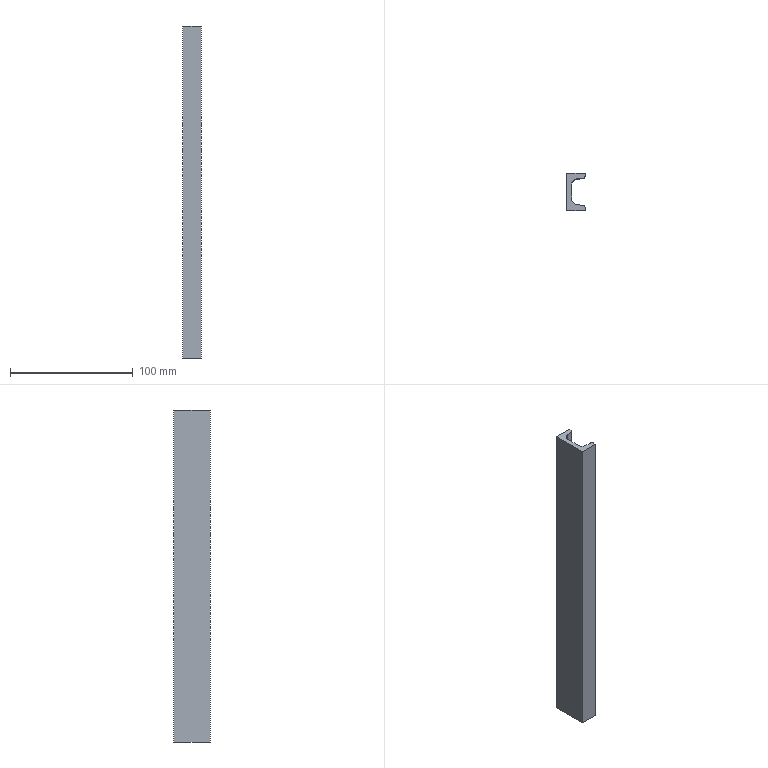Part | STEP file | DIN 1026-1 U 30x15 1785507675476 | 1 solid | 14 faces | box 15 x 30 x 270 mm | volume 59739 mm3 | plane 10 | cylinder 4 | commonest cylinder face diameters 4 x2 9 x2
STEP:
#1=CARTESIAN_POINT('',(4.,-6.066,270.));
#2=VERTEX_POINT('',#1);
#3=CARTESIAN_POINT('',(8.141,-10.551,270.));
#4=VERTEX_POINT('',#3);
#5=CARTESIAN_POINT('',(8.5,-6.066,270.));
#6=DIRECTION('',(0.,0.,1.));
#7=DIRECTION('',(-1.,0.,0.));
#8=AXIS2_PLACEMENT_3D('',#5,#6,#7);
#9=CIRCLE('',#8,4.5);
#10=EDGE_CURVE('',#2,#4,#9,.T.);
#11=ORIENTED_EDGE('',*,*,#10,.T.);
#12=CARTESIAN_POINT('',(8.141,-10.551,0.));
#13=VERTEX_POINT('',#12);
#14=CARTESIAN_POINT('',(8.141,-10.551,0.));
#15=DIRECTION('',(0.,0.,1.));
#16=VECTOR('',#15,10.);
#17=LINE('',#14,#16);
#18=EDGE_CURVE('',#13,#4,#17,.T.);
#19=ORIENTED_EDGE('',*,*,#18,.F.);
#20=CARTESIAN_POINT('',(4.,-6.066,0.));
#21=VERTEX_POINT('',#20);
#22=CARTESIAN_POINT('',(8.5,-6.066,0.));
#23=DIRECTION('',(0.,0.,1.));
#24=DIRECTION('',(-1.,0.,0.));
#25=AXIS2_PLACEMENT_3D('',#22,#23,#24);
#26=CIRCLE('',#25,4.5);
#27=EDGE_CURVE('',#21,#13,#26,.T.);
#28=ORIENTED_EDGE('',*,*,#27,.F.);
#29=CARTESIAN_POINT('',(4.,-6.066,0.));
#30=DIRECTION('',(0.,0.,1.));
#31=VECTOR('',#30,10.);
#32=LINE('',#29,#31);
#33=EDGE_CURVE('',#21,#2,#32,.T.);
#34=ORIENTED_EDGE('',*,*,#33,.T.);
#35=EDGE_LOOP('',(#11,#19,#28,#34));
#36=FACE_OUTER_BOUND('',#35,.T.);
#37=CARTESIAN_POINT('',(8.5,-6.066,0.));
#38=DIRECTION('',(0.,0.,1.));
#39=DIRECTION('',(-1.,0.,0.));
#40=AXIS2_PLACEMENT_3D('',#37,#38,#39);
#41=CYLINDRICAL_SURFACE('',#40,4.5);
#42=ADVANCED_FACE('',(#36),#41,.F.);
#43=CARTESIAN_POINT('',(13.159,-10.953,270.));
#44=VERTEX_POINT('',#43);
#45=CARTESIAN_POINT('',(7.403,-10.492,270.));
#46=DIRECTION('',(0.9968,-0.07975,0.));
#47=VECTOR('',#46,10.);
#48=LINE('',#45,#47);
#49=EDGE_CURVE('',#4,#44,#48,.T.);
#50=ORIENTED_EDGE('',*,*,#49,.T.);
#51=CARTESIAN_POINT('',(13.159,-10.953,0.));
#52=VERTEX_POINT('',#51);
#53=CARTESIAN_POINT('',(13.159,-10.953,0.));
#54=DIRECTION('',(0.,0.,1.));
#55=VECTOR('',#54,10.);
#56=LINE('',#53,#55);
#57=EDGE_CURVE('',#52,#44,#56,.T.);
#58=ORIENTED_EDGE('',*,*,#57,.F.);
#59=CARTESIAN_POINT('',(7.403,-10.492,0.));
#60=DIRECTION('',(0.9968,-0.07975,0.));
#61=VECTOR('',#60,10.);
#62=LINE('',#59,#61);
#63=EDGE_CURVE('',#13,#52,#62,.T.);
#64=ORIENTED_EDGE('',*,*,#63,.F.);
#65=ORIENTED_EDGE('',*,*,#18,.T.);
#66=EDGE_LOOP('',(#50,#58,#64,#65));
#67=FACE_OUTER_BOUND('',#66,.T.);
#68=CARTESIAN_POINT('',(8.141,-10.551,0.));
#69=DIRECTION('',(0.07975,0.9968,0.));
#70=DIRECTION('',(0.,0.,1.));
#71=AXIS2_PLACEMENT_3D('',#68,#69,#70);
#72=PLANE('',#71);
#73=ADVANCED_FACE('',(#67),#72,.T.);
#74=CARTESIAN_POINT('',(15.,-12.946,270.));
#75=VERTEX_POINT('',#74);
#76=CARTESIAN_POINT('',(13.,-12.946,270.));
#77=DIRECTION('',(0.,0.,-1.));
#78=DIRECTION('',(-1.,0.,0.));
#79=AXIS2_PLACEMENT_3D('',#76,#77,#78);
#80=CIRCLE('',#79,2.);
#81=EDGE_CURVE('',#44,#75,#80,.T.);
#82=ORIENTED_EDGE('',*,*,#81,.T.);
#83=CARTESIAN_POINT('',(15.,-12.946,0.));
#84=VERTEX_POINT('',#83);
#85=CARTESIAN_POINT('',(15.,-12.946,0.));
#86=DIRECTION('',(0.,0.,1.));
#87=VECTOR('',#86,10.);
#88=LINE('',#85,#87);
#89=EDGE_CURVE('',#84,#75,#88,.T.);
#90=ORIENTED_EDGE('',*,*,#89,.F.);
#91=CARTESIAN_POINT('',(13.,-12.946,0.));
#92=DIRECTION('',(0.,0.,-1.));
#93=DIRECTION('',(-1.,0.,0.));
#94=AXIS2_PLACEMENT_3D('',#91,#92,#93);
#95=CIRCLE('',#94,2.);
#96=EDGE_CURVE('',#52,#84,#95,.T.);
#97=ORIENTED_EDGE('',*,*,#96,.F.);
#98=ORIENTED_EDGE('',*,*,#57,.T.);
#99=EDGE_LOOP('',(#82,#90,#97,#98));
#100=FACE_OUTER_BOUND('',#99,.T.);
#101=CARTESIAN_POINT('',(13.,-12.946,0.));
#102=DIRECTION('',(0.,0.,1.));
#103=DIRECTION('',(-1.,0.,0.));
#104=AXIS2_PLACEMENT_3D('',#101,#102,#103);
#105=CYLINDRICAL_SURFACE('',#104,2.);
#106=ADVANCED_FACE('',(#100),#105,.T.);
#107=CARTESIAN_POINT('',(15.,-15.,270.));
#108=VERTEX_POINT('',#107);
#109=CARTESIAN_POINT('',(15.,-6.473,270.));
#110=DIRECTION('',(0.,-1.,0.));
#111=VECTOR('',#110,10.);
#112=LINE('',#109,#111);
#113=EDGE_CURVE('',#75,#108,#112,.T.);
#114=ORIENTED_EDGE('',*,*,#113,.T.);
#115=CARTESIAN_POINT('',(15.,-15.,0.));
#116=VERTEX_POINT('',#115);
#117=CARTESIAN_POINT('',(15.,-15.,0.));
#118=DIRECTION('',(0.,0.,1.));
#119=VECTOR('',#118,10.);
#120=LINE('',#117,#119);
#121=EDGE_CURVE('',#116,#108,#120,.T.);
#122=ORIENTED_EDGE('',*,*,#121,.F.);
#123=CARTESIAN_POINT('',(15.,-6.473,0.));
#124=DIRECTION('',(0.,-1.,0.));
#125=VECTOR('',#124,10.);
#126=LINE('',#123,#125);
#127=EDGE_CURVE('',#84,#116,#126,.T.);
#128=ORIENTED_EDGE('',*,*,#127,.F.);
#129=ORIENTED_EDGE('',*,*,#89,.T.);
#130=EDGE_LOOP('',(#114,#122,#128,#129));
#131=FACE_OUTER_BOUND('',#130,.T.);
#132=CARTESIAN_POINT('',(15.,-12.946,0.));
#133=DIRECTION('',(1.,0.,0.));
#134=DIRECTION('',(0.,0.,-1.));
#135=AXIS2_PLACEMENT_3D('',#132,#133,#134);
#136=PLANE('',#135);
#137=ADVANCED_FACE('',(#131),#136,.T.);
#138=CARTESIAN_POINT('',(0.,-15.,270.));
#139=VERTEX_POINT('',#138);
#140=CARTESIAN_POINT('',(11.25,-15.,270.));
#141=DIRECTION('',(-1.,0.,0.));
#142=VECTOR('',#141,10.);
#143=LINE('',#140,#142);
#144=EDGE_CURVE('',#108,#139,#143,.T.);
#145=ORIENTED_EDGE('',*,*,#144,.T.);
#146=CARTESIAN_POINT('',(0.,-15.,0.));
#147=VERTEX_POINT('',#146);
#148=CARTESIAN_POINT('',(0.,-15.,0.));
#149=DIRECTION('',(0.,0.,1.));
#150=VECTOR('',#149,10.);
#151=LINE('',#148,#150);
#152=EDGE_CURVE('',#147,#139,#151,.T.);
#153=ORIENTED_EDGE('',*,*,#152,.F.);
#154=CARTESIAN_POINT('',(11.25,-15.,0.));
#155=DIRECTION('',(-1.,0.,0.));
#156=VECTOR('',#155,10.);
#157=LINE('',#154,#156);
#158=EDGE_CURVE('',#116,#147,#157,.T.);
#159=ORIENTED_EDGE('',*,*,#158,.F.);
#160=ORIENTED_EDGE('',*,*,#121,.T.);
#161=EDGE_LOOP('',(#145,#153,#159,#160));
#162=FACE_OUTER_BOUND('',#161,.T.);
#163=CARTESIAN_POINT('',(15.,-15.,0.));
#164=DIRECTION('',(0.,-1.,0.));
#165=DIRECTION('',(0.,0.,-1.));
#166=AXIS2_PLACEMENT_3D('',#163,#164,#165);
#167=PLANE('',#166);
#168=ADVANCED_FACE('',(#162),#167,.T.);
#169=CARTESIAN_POINT('',(0.,15.,270.));
#170=VERTEX_POINT('',#169);
#171=CARTESIAN_POINT('',(0.,0.,270.));
#172=DIRECTION('',(0.,1.,0.));
#173=VECTOR('',#172,10.);
#174=LINE('',#171,#173);
#175=EDGE_CURVE('',#139,#170,#174,.T.);
#176=ORIENTED_EDGE('',*,*,#175,.T.);
#177=CARTESIAN_POINT('',(0.,15.,0.));
#178=VERTEX_POINT('',#177);
#179=CARTESIAN_POINT('',(0.,15.,0.));
#180=DIRECTION('',(0.,0.,1.));
#181=VECTOR('',#180,10.);
#182=LINE('',#179,#181);
#183=EDGE_CURVE('',#178,#170,#182,.T.);
#184=ORIENTED_EDGE('',*,*,#183,.F.);
#185=CARTESIAN_POINT('',(0.,0.,0.));
#186=DIRECTION('',(0.,1.,0.));
#187=VECTOR('',#186,10.);
#188=LINE('',#185,#187);
#189=EDGE_CURVE('',#147,#178,#188,.T.);
#190=ORIENTED_EDGE('',*,*,#189,.F.);
#191=ORIENTED_EDGE('',*,*,#152,.T.);
#192=EDGE_LOOP('',(#176,#184,#190,#191));
#193=FACE_OUTER_BOUND('',#192,.T.);
#194=CARTESIAN_POINT('',(0.,0.,0.));
#195=DIRECTION('',(-1.,0.,0.));
#196=DIRECTION('',(0.,0.,1.));
#197=AXIS2_PLACEMENT_3D('',#194,#195,#196);
#198=PLANE('',#197);
#199=ADVANCED_FACE('',(#193),#198,.T.);
#200=CARTESIAN_POINT('',(15.,15.,270.));
#201=VERTEX_POINT('',#200);
#202=CARTESIAN_POINT('',(3.75,15.,270.));
#203=DIRECTION('',(1.,0.,0.));
#204=VECTOR('',#203,10.);
#205=LINE('',#202,#204);
#206=EDGE_CURVE('',#170,#201,#205,.T.);
#207=ORIENTED_EDGE('',*,*,#206,.T.);
#208=CARTESIAN_POINT('',(15.,15.,0.));
#209=VERTEX_POINT('',#208);
#210=CARTESIAN_POINT('',(15.,15.,0.));
#211=DIRECTION('',(0.,0.,1.));
#212=VECTOR('',#211,10.);
#213=LINE('',#210,#212);
#214=EDGE_CURVE('',#209,#201,#213,.T.);
#215=ORIENTED_EDGE('',*,*,#214,.F.);
#216=CARTESIAN_POINT('',(3.75,15.,0.));
#217=DIRECTION('',(1.,0.,0.));
#218=VECTOR('',#217,10.);
#219=LINE('',#216,#218);
#220=EDGE_CURVE('',#178,#209,#219,.T.);
#221=ORIENTED_EDGE('',*,*,#220,.F.);
#222=ORIENTED_EDGE('',*,*,#183,.T.);
#223=EDGE_LOOP('',(#207,#215,#221,#222));
#224=FACE_OUTER_BOUND('',#223,.T.);
#225=CARTESIAN_POINT('',(0.,15.,0.));
#226=DIRECTION('',(0.,1.,0.));
#227=DIRECTION('',(0.,0.,1.));
#228=AXIS2_PLACEMENT_3D('',#225,#226,#227);
#229=PLANE('',#228);
#230=ADVANCED_FACE('',(#224),#229,.T.);
#231=CARTESIAN_POINT('',(15.,12.946,270.));
#232=VERTEX_POINT('',#231);
#233=CARTESIAN_POINT('',(15.,7.5,270.));
#234=DIRECTION('',(0.,-1.,0.));
#235=VECTOR('',#234,10.);
#236=LINE('',#233,#235);
#237=EDGE_CURVE('',#201,#232,#236,.T.);
#238=ORIENTED_EDGE('',*,*,#237,.T.);
#239=CARTESIAN_POINT('',(15.,12.946,0.));
#240=VERTEX_POINT('',#239);
#241=CARTESIAN_POINT('',(15.,12.946,0.));
#242=DIRECTION('',(0.,0.,1.));
#243=VECTOR('',#242,10.);
#244=LINE('',#241,#243);
#245=EDGE_CURVE('',#240,#232,#244,.T.);
#246=ORIENTED_EDGE('',*,*,#245,.F.);
#247=CARTESIAN_POINT('',(15.,7.5,0.));
#248=DIRECTION('',(0.,-1.,0.));
#249=VECTOR('',#248,10.);
#250=LINE('',#247,#249);
#251=EDGE_CURVE('',#209,#240,#250,.T.);
#252=ORIENTED_EDGE('',*,*,#251,.F.);
#253=ORIENTED_EDGE('',*,*,#214,.T.);
#254=EDGE_LOOP('',(#238,#246,#252,#253));
#255=FACE_OUTER_BOUND('',#254,.T.);
#256=CARTESIAN_POINT('',(15.,15.,0.));
#257=DIRECTION('',(1.,0.,0.));
#258=DIRECTION('',(0.,0.,-1.));
#259=AXIS2_PLACEMENT_3D('',#256,#257,#258);
#260=PLANE('',#259);
#261=ADVANCED_FACE('',(#255),#260,.T.);
#262=CARTESIAN_POINT('',(13.159,10.953,270.));
#263=VERTEX_POINT('',#262);
#264=CARTESIAN_POINT('',(13.,12.946,270.));
#265=DIRECTION('',(0.,0.,-1.));
#266=DIRECTION('',(-0.07975,0.9968,0.));
#267=AXIS2_PLACEMENT_3D('',#264,#265,#266);
#268=CIRCLE('',#267,2.);
#269=EDGE_CURVE('',#232,#263,#268,.T.);
#270=ORIENTED_EDGE('',*,*,#269,.T.);
#271=CARTESIAN_POINT('',(13.159,10.953,0.));
#272=VERTEX_POINT('',#271);
#273=CARTESIAN_POINT('',(13.159,10.953,0.));
#274=DIRECTION('',(0.,0.,1.));
#275=VECTOR('',#274,10.);
#276=LINE('',#273,#275);
#277=EDGE_CURVE('',#272,#263,#276,.T.);
#278=ORIENTED_EDGE('',*,*,#277,.F.);
#279=CARTESIAN_POINT('',(13.,12.946,0.));
#280=DIRECTION('',(0.,0.,-1.));
#281=DIRECTION('',(-0.07975,0.9968,0.));
#282=AXIS2_PLACEMENT_3D('',#279,#280,#281);
#283=CIRCLE('',#282,2.);
#284=EDGE_CURVE('',#240,#272,#283,.T.);
#285=ORIENTED_EDGE('',*,*,#284,.F.);
#286=ORIENTED_EDGE('',*,*,#245,.T.);
#287=EDGE_LOOP('',(#270,#278,#285,#286));
#288=FACE_OUTER_BOUND('',#287,.T.);
#289=CARTESIAN_POINT('',(13.,12.946,0.));
#290=DIRECTION('',(0.,0.,1.));
#291=DIRECTION('',(-0.07975,0.9968,0.));
#292=AXIS2_PLACEMENT_3D('',#289,#290,#291);
#293=CYLINDRICAL_SURFACE('',#292,2.);
#294=ADVANCED_FACE('',(#288),#293,.T.);
#295=CARTESIAN_POINT('',(8.141,10.551,270.));
#296=VERTEX_POINT('',#295);
#297=CARTESIAN_POINT('',(9.912,10.693,270.));
#298=DIRECTION('',(-0.9968,-0.07975,0.));
#299=VECTOR('',#298,10.);
#300=LINE('',#297,#299);
#301=EDGE_CURVE('',#263,#296,#300,.T.);
#302=ORIENTED_EDGE('',*,*,#301,.T.);
#303=CARTESIAN_POINT('',(8.141,10.551,0.));
#304=VERTEX_POINT('',#303);
#305=CARTESIAN_POINT('',(8.141,10.551,0.));
#306=DIRECTION('',(0.,0.,1.));
#307=VECTOR('',#306,10.);
#308=LINE('',#305,#307);
#309=EDGE_CURVE('',#304,#296,#308,.T.);
#310=ORIENTED_EDGE('',*,*,#309,.F.);
#311=CARTESIAN_POINT('',(9.912,10.693,0.));
#312=DIRECTION('',(-0.9968,-0.07975,0.));
#313=VECTOR('',#312,10.);
#314=LINE('',#311,#313);
#315=EDGE_CURVE('',#272,#304,#314,.T.);
#316=ORIENTED_EDGE('',*,*,#315,.F.);
#317=ORIENTED_EDGE('',*,*,#277,.T.);
#318=EDGE_LOOP('',(#302,#310,#316,#317));
#319=FACE_OUTER_BOUND('',#318,.T.);
#320=CARTESIAN_POINT('',(13.159,10.953,0.));
#321=DIRECTION('',(0.07975,-0.9968,0.));
#322=DIRECTION('',(0.,0.,-1.));
#323=AXIS2_PLACEMENT_3D('',#320,#321,#322);
#324=PLANE('',#323);
#325=ADVANCED_FACE('',(#319),#324,.T.);
#326=CARTESIAN_POINT('',(4.,6.066,270.));
#327=VERTEX_POINT('',#326);
#328=CARTESIAN_POINT('',(8.5,6.066,270.));
#329=DIRECTION('',(0.,0.,1.));
#330=DIRECTION('',(-0.07975,0.9968,0.));
#331=AXIS2_PLACEMENT_3D('',#328,#329,#330);
#332=CIRCLE('',#331,4.5);
#333=EDGE_CURVE('',#296,#327,#332,.T.);
#334=ORIENTED_EDGE('',*,*,#333,.T.);
#335=CARTESIAN_POINT('',(4.,6.066,0.));
#336=VERTEX_POINT('',#335);
#337=CARTESIAN_POINT('',(4.,6.066,0.));
#338=DIRECTION('',(0.,0.,1.));
#339=VECTOR('',#338,10.);
#340=LINE('',#337,#339);
#341=EDGE_CURVE('',#336,#327,#340,.T.);
#342=ORIENTED_EDGE('',*,*,#341,.F.);
#343=CARTESIAN_POINT('',(8.5,6.066,0.));
#344=DIRECTION('',(0.,0.,1.));
#345=DIRECTION('',(-0.07975,0.9968,0.));
#346=AXIS2_PLACEMENT_3D('',#343,#344,#345);
#347=CIRCLE('',#346,4.5);
#348=EDGE_CURVE('',#304,#336,#347,.T.);
#349=ORIENTED_EDGE('',*,*,#348,.F.);
#350=ORIENTED_EDGE('',*,*,#309,.T.);
#351=EDGE_LOOP('',(#334,#342,#349,#350));
#352=FACE_OUTER_BOUND('',#351,.T.);
#353=CARTESIAN_POINT('',(8.5,6.066,0.));
#354=DIRECTION('',(0.,0.,1.));
#355=DIRECTION('',(-0.07975,0.9968,0.));
#356=AXIS2_PLACEMENT_3D('',#353,#354,#355);
#357=CYLINDRICAL_SURFACE('',#356,4.5);
#358=ADVANCED_FACE('',(#352),#357,.F.);
#359=CARTESIAN_POINT('',(4.,0.,270.));
#360=DIRECTION('',(0.,-1.,0.));
#361=VECTOR('',#360,10.);
#362=LINE('',#359,#361);
#363=EDGE_CURVE('',#327,#2,#362,.T.);
#364=ORIENTED_EDGE('',*,*,#363,.T.);
#365=ORIENTED_EDGE('',*,*,#33,.F.);
#366=CARTESIAN_POINT('',(4.,0.,0.));
#367=DIRECTION('',(0.,-1.,0.));
#368=VECTOR('',#367,10.);
#369=LINE('',#366,#368);
#370=EDGE_CURVE('',#336,#21,#369,.T.);
#371=ORIENTED_EDGE('',*,*,#370,.F.);
#372=ORIENTED_EDGE('',*,*,#341,.T.);
#373=EDGE_LOOP('',(#364,#365,#371,#372));
#374=FACE_OUTER_BOUND('',#373,.T.);
#375=CARTESIAN_POINT('',(4.,0.,0.));
#376=DIRECTION('',(1.,0.,0.));
#377=DIRECTION('',(0.,0.,-1.));
#378=AXIS2_PLACEMENT_3D('',#375,#376,#377);
#379=PLANE('',#378);
#380=ADVANCED_FACE('',(#374),#379,.T.);
#381=ORIENTED_EDGE('',*,*,#220,.T.);
#382=ORIENTED_EDGE('',*,*,#251,.T.);
#383=ORIENTED_EDGE('',*,*,#284,.T.);
#384=ORIENTED_EDGE('',*,*,#315,.T.);
#385=ORIENTED_EDGE('',*,*,#348,.T.);
#386=ORIENTED_EDGE('',*,*,#370,.T.);
#387=ORIENTED_EDGE('',*,*,#27,.T.);
#388=ORIENTED_EDGE('',*,*,#63,.T.);
#389=ORIENTED_EDGE('',*,*,#96,.T.);
#390=ORIENTED_EDGE('',*,*,#127,.T.);
#391=ORIENTED_EDGE('',*,*,#158,.T.);
#392=ORIENTED_EDGE('',*,*,#189,.T.);
#393=EDGE_LOOP('',(#381,#382,#383,#384,#385,#386,#387,#388,#389,#390,#391,#392));
#394=FACE_OUTER_BOUND('',#393,.T.);
#395=CARTESIAN_POINT('',(7.5,0.,0.));
#396=DIRECTION('',(0.,0.,1.));
#397=DIRECTION('',(1.,0.,0.));
#398=AXIS2_PLACEMENT_3D('',#395,#396,#397);
#399=PLANE('',#398);
#400=ADVANCED_FACE('',(#394),#399,.F.);
#401=ORIENTED_EDGE('',*,*,#206,.F.);
#402=ORIENTED_EDGE('',*,*,#175,.F.);
#403=ORIENTED_EDGE('',*,*,#144,.F.);
#404=ORIENTED_EDGE('',*,*,#113,.F.);
#405=ORIENTED_EDGE('',*,*,#81,.F.);
#406=ORIENTED_EDGE('',*,*,#49,.F.);
#407=ORIENTED_EDGE('',*,*,#10,.F.);
#408=ORIENTED_EDGE('',*,*,#363,.F.);
#409=ORIENTED_EDGE('',*,*,#333,.F.);
#410=ORIENTED_EDGE('',*,*,#301,.F.);
#411=ORIENTED_EDGE('',*,*,#269,.F.);
#412=ORIENTED_EDGE('',*,*,#237,.F.);
#413=EDGE_LOOP('',(#401,#402,#403,#404,#405,#406,#407,#408,#409,#410,#411,#412));
#414=FACE_OUTER_BOUND('',#413,.T.);
#415=CARTESIAN_POINT('',(7.5,0.,270.));
#416=DIRECTION('',(0.,0.,1.));
#417=DIRECTION('',(1.,0.,0.));
#418=AXIS2_PLACEMENT_3D('',#415,#416,#417);
#419=PLANE('',#418);
#420=ADVANCED_FACE('',(#414),#419,.T.);
#421=CLOSED_SHELL('',(#42,#73,#106,#137,#168,#199,#230,#261,#294,#325,#358,#380,#400,#420));
#422=MANIFOLD_SOLID_BREP('',#421);
#423=(LENGTH_UNIT()NAMED_UNIT(*)SI_UNIT(.MILLI.,.METRE.));
#424=UNCERTAINTY_MEASURE_WITH_UNIT(LENGTH_MEASURE(0.01),#423,'','');
#425=(NAMED_UNIT(*)PLANE_ANGLE_UNIT()SI_UNIT($,.RADIAN.));
#426=(NAMED_UNIT(*)SI_UNIT($,.STERADIAN.)SOLID_ANGLE_UNIT());
#427=(GEOMETRIC_REPRESENTATION_CONTEXT(3)GLOBAL_UNCERTAINTY_ASSIGNED_CONTEXT((#424))GLOBAL_UNIT_ASSIGNED_CONTEXT((#423,#425,#426))REPRESENTATION_CONTEXT('',''));
#428=ADVANCED_BREP_SHAPE_REPRESENTATION('',(#422),#427);